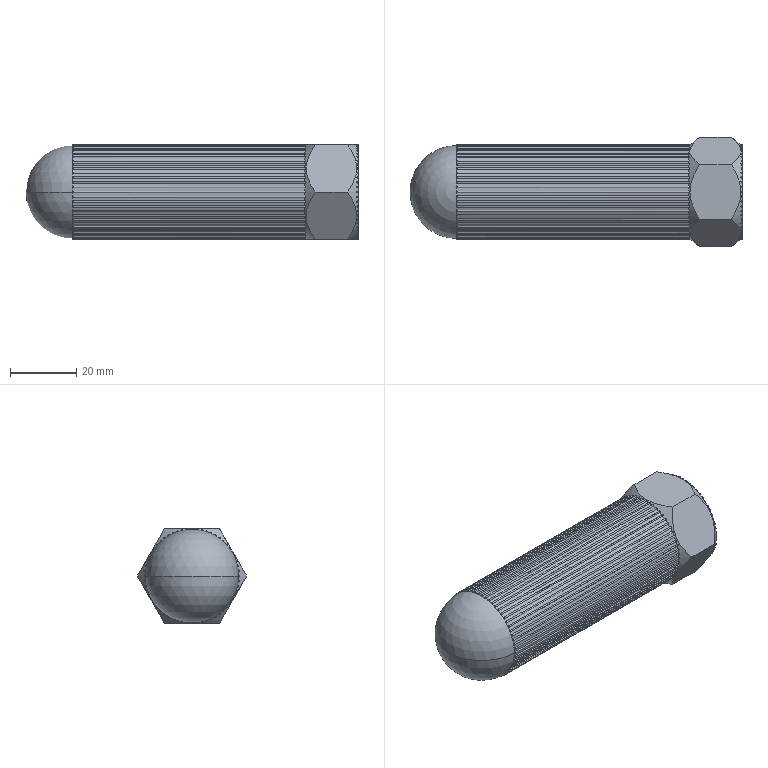Part | SolidWorks | features BaseBody 1 | 1 solid | 680 faces | box 100 x 32.95 x 28.536 mm | volume 29747 mm3 | cylinder 424 | torus 180 | plane 68 | cone 6 | sphere 2 | commonest cylinder face diameters 0.5 x360 28 x60 17.294 x2 21.6 x2